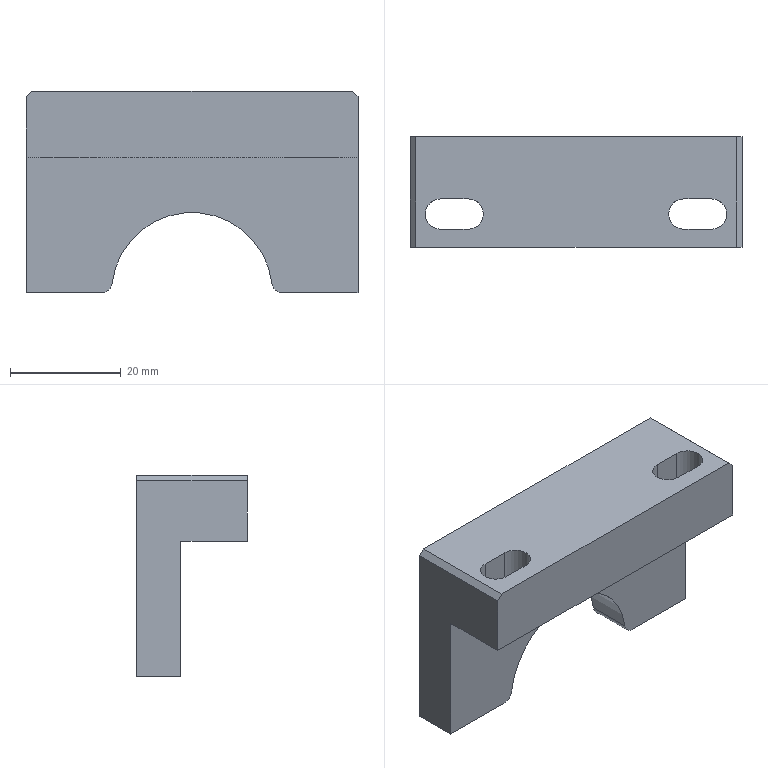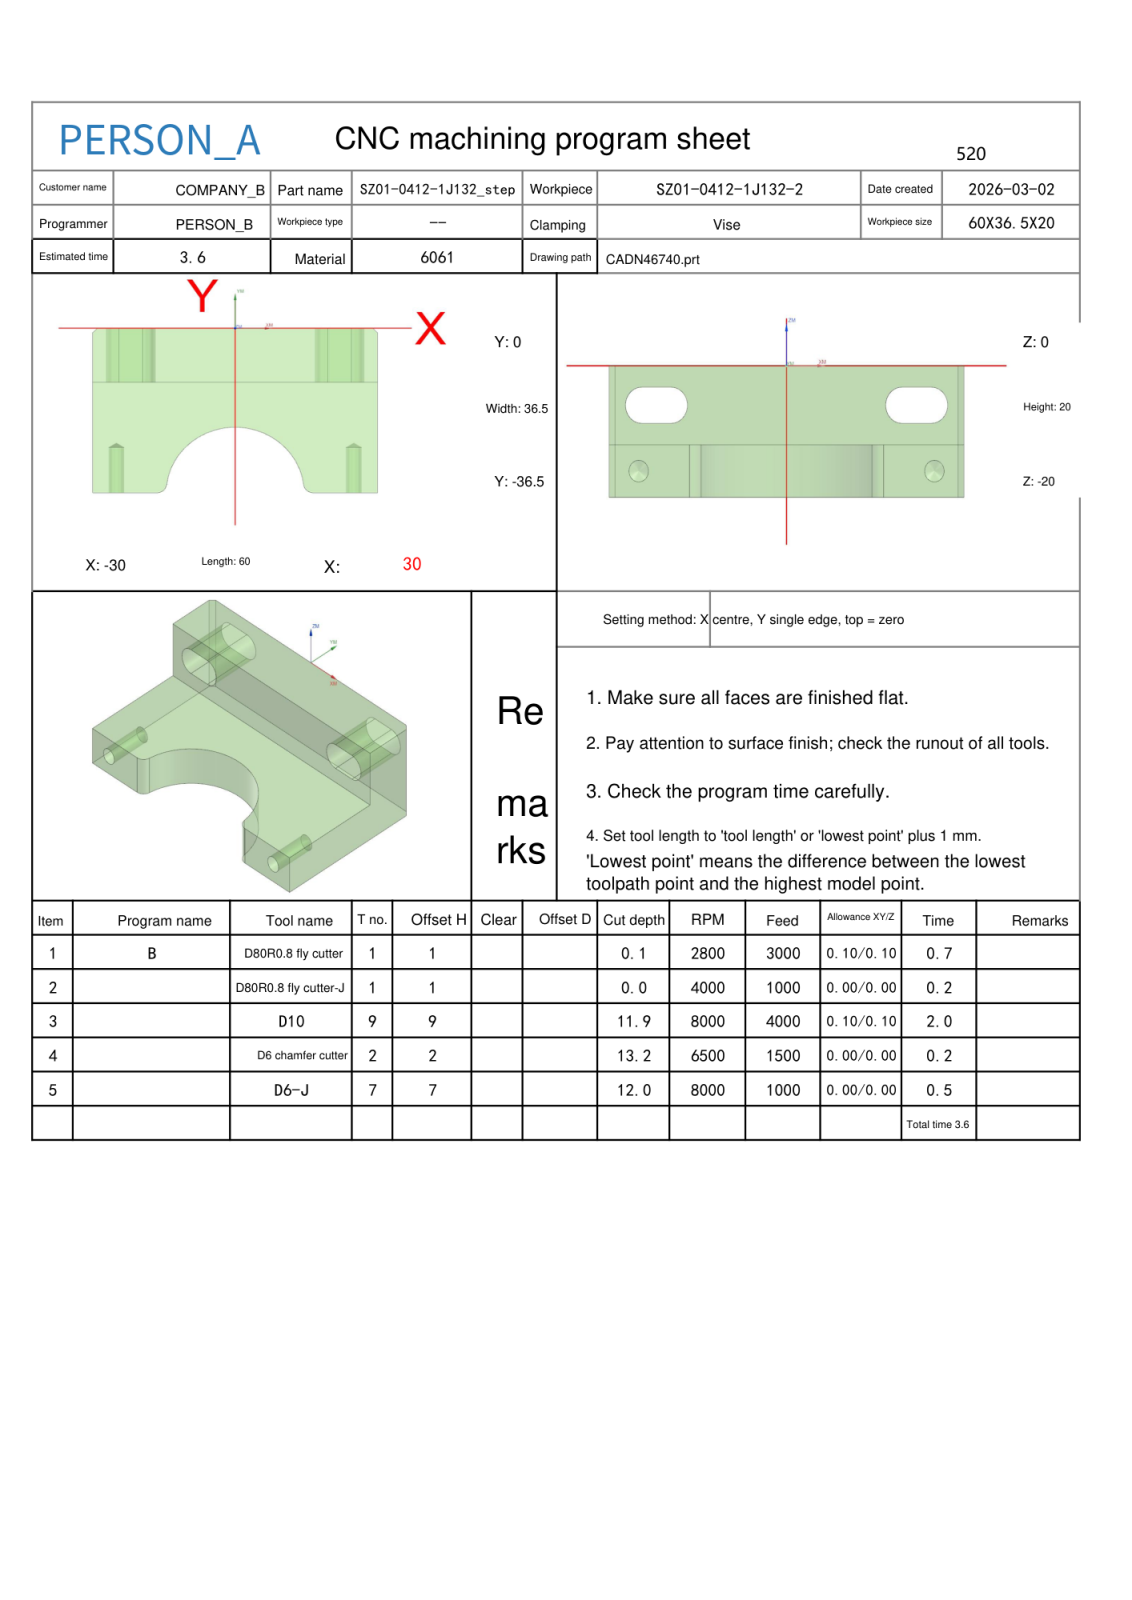NC program | NX | posted by the shop | part box 60 x 20 x 36.5 mm
Whole program, first 1625 of 1831 lines:
%
O0001
(Machine time: 4.61 MIN)
(===Total Tool:4===)
(T1=D80R0.8 fly cutter D=80.  R=0.8  D-  H01 Z=0.    )
(T9=D10     D=10.  R=0.   D-  H09 Z=-11.9 )
(T2=D6 chamfer cutter   D=6.   R=0.   D-  H02 Z=-13.2 )
(T7=D6-J    D=6.   R=0.   D7  H07 Z=-12.  )
G80 G90 G17 G49 G40
G91 G28 Z0
M01
N1 T01 M06
(D80R0.8 fly cutter  D=80. R=0.8 H=01 ce=0.10 di=0.10)
G00 G90 G54 X82.097 Y-18.25 M03 S2800
G43 H01 Z50.
M08
Z6.011
G01 Z4.011 F3000.
X70.097
X-70.097
X-82.097
Z6.011
G00 X82.097
Z5.522
G01 Z3.522
X70.097
X-70.097
X-82.097
Z5.522
G00 X82.097
Z5.033
G01 Z3.033
X70.097
X-70.097
X-82.097
Z5.033
G00 X82.097
Z4.544
G01 Z2.544
X70.097
X-70.097
X-82.097
Z4.544
G00 Z50.
X82.097
Z4.056
G01 Z2.056
X70.097
X-70.097
X-82.097
Z4.056
G00 Z50.
X82.097
Z3.567
G01 Z1.567
X70.097
X-70.097
X-82.097
Z3.567
G00 Z50.
X82.097
Z3.078
G01 Z1.078
X70.097
X-70.097
X-82.097
Z3.078
G00 Z50.
X82.097
Z2.589
G01 Z.589
X70.097
X-70.097
X-82.097
Z2.589
G00 Z50.
X82.097
Z2.1
G01 Z.1
X70.097
X-70.097
X-82.097
Z2.1
G00 Z50.
G91 G28 Z0.0
M05
M09
G91 G28 Z0.0
M01
N2 T01 M06
(D80R0.8 fly cutter-J  D=80. R=0.8 H=01 ce=0.00 di=0.00)
G00 G90 G54 X81.999 Y-18.25 M03 S4000
G43 H01 Z50.
M08
Z2.
G01 Z0.0 F1000.
X69.999
X-69.999
X-81.999
Z2.
G00 Z50.
G91 G28 Z0.0
M05
M09
G91 G28 Z0.0
M01
N3 T09 M06
(D10  D=10. R=0. H=09 ce=0.10 di=0.10)
G00 G90 G54 X38. Y-29.25 M03 S8000
G43 H09 Z14.5
M08
Z.905
G01 Z-.595 F4000.
X34.9
Y-41.4
X16.429
G02 X9.579 Y-35.334 I0.0 J6.9
G03 X0.0 Y-26.85 I-9.579 J-1.166
X-9.579 Y-35.334 I0.0 J-9.65
G02 X-16.429 Y-41.4 I-6.849 J.834
G01 X-34.9
Y-17.1
X-14.511
G02 X-13.511 Y-18.1 I0.0 J-1.
G01 X-13.522 Y-18.254
X-14.384 Y-23.787
X-14.396 Y-23.941
G03 X-13.954 Y-24.77 I1. J0.0
G02 X-13.512 Y-25.6 I-.558 J-.83
X-13.712 Y-26.199 I-1. J0.0
G03 X-16.81 Y-33.1 I13.712 J-10.301
G02 X-17.787 Y-33.9 I-.98 J.2
G01 X-26.402
G02 X-27.4 Y-32.902 I.002 J1.
G01 Y-25.598
G02 X-26.402 Y-24.6 I1. J-.002
G01 X-17.809
G03 X-16.834 Y-23.822 I0.0 J1.
G01 X-15.486 Y-17.879
G02 X-14.511 Y-17.1 I.975 J-.221
G01 X-.81
G02 X.189 Y-18.066 I0.0 J-1.
G01 X.205 Y-18.539
G03 X.764 Y-19.403 I.999 J.034
G02 X2.162 Y-21.647 I-1.102 J-2.244
X.134 Y-24.102 I-2.5 J0.0
G01 X-10.853 Y-26.214
G02 X-11.325 Y-26.259 I-.472 J2.455
X-13.825 Y-23.759 I0.0 J2.5
X-11.797 Y-21.304 I2.5 J0.0
G01 X-2.631 Y-19.542
G03 X-1.82 Y-18.581 I-.189 J.982
G01 X-1.81 Y-18.079
G02 X-.81 Y-17.1 I1. J-.021
G01 X.81
G02 X1.81 Y-18.079 I0.0 J-1.
G01 X1.82 Y-18.581
G03 X2.631 Y-19.542 I1. J.021
G01 X11.797 Y-21.304
G02 X13.825 Y-23.759 I-.472 J-2.455
X11.325 Y-26.259 I-2.5 J0.0
X10.853 Y-26.214 I0.0 J2.5
G01 X-.134 Y-24.102
G02 X-2.162 Y-21.647 I.472 J2.455
X-.764 Y-19.403 I2.5 J0.0
G03 X-.205 Y-18.539 I-.441 J.897
G01 X-.189 Y-18.066
G02 X.81 Y-17.1 I.999 J-.034
G01 X34.9
Y-26.215
G02 X34.455 Y-27.047 I-1. J0.0
G01 X27.845 Y-31.453
G03 X27.4 Y-32.285 I.555 J-.832
G01 Y-32.902
G02 X26.402 Y-33.9 I-1. J.002
G01 X17.787
G02 X16.81 Y-33.1 I.002 J1.
G03 X13.712 Y-26.199 I-16.81 J-3.4
G02 X13.512 Y-25.6 I.801 J.599
X14.511 Y-24.6 I1. J0.0
G01 X26.402
G02 X27.4 Y-25.598 I-.002 J-1.
G01 Y-29.25
Y-29.75
X38.
Z.905
G00 Y-29.25
Z.31
G01 Z-1.19
X34.9
Y-41.4
X16.429
G02 X9.579 Y-35.334 I0.0 J6.9
G03 X0.0 Y-26.85 I-9.579 J-1.166
X-9.579 Y-35.334 I0.0 J-9.65
G02 X-16.429 Y-41.4 I-6.849 J.834
G01 X-34.9
Y-17.1
X-14.511
G02 X-13.511 Y-18.1 I0.0 J-1.
G01 X-13.522 Y-18.254
X-14.384 Y-23.787
X-14.396 Y-23.941
G03 X-13.954 Y-24.77 I1. J0.0
G02 X-13.512 Y-25.6 I-.558 J-.83
X-13.712 Y-26.199 I-1. J0.0
G03 X-16.81 Y-33.1 I13.712 J-10.301
G02 X-17.787 Y-33.9 I-.98 J.2
G01 X-26.402
G02 X-27.4 Y-32.902 I.002 J1.
G01 Y-25.598
G02 X-26.402 Y-24.6 I1. J-.002
G01 X-17.809
G03 X-16.834 Y-23.822 I0.0 J1.
G01 X-15.486 Y-17.879
G02 X-14.511 Y-17.1 I.975 J-.221
G01 X-.81
G02 X.189 Y-18.066 I0.0 J-1.
G01 X.205 Y-18.539
G03 X.764 Y-19.403 I.999 J.034
G02 X2.162 Y-21.647 I-1.102 J-2.244
X.134 Y-24.102 I-2.5 J0.0
G01 X-10.853 Y-26.214
G02 X-11.325 Y-26.259 I-.472 J2.455
X-13.825 Y-23.759 I0.0 J2.5
X-11.797 Y-21.304 I2.5 J0.0
G01 X-2.631 Y-19.542
G03 X-1.82 Y-18.581 I-.189 J.982
G01 X-1.81 Y-18.079
G02 X-.81 Y-17.1 I1. J-.021
G01 X.81
G02 X1.81 Y-18.079 I0.0 J-1.
G01 X1.82 Y-18.581
G03 X2.631 Y-19.542 I1. J.021
G01 X11.797 Y-21.304
G02 X13.825 Y-23.759 I-.472 J-2.455
X11.325 Y-26.259 I-2.5 J0.0
X10.853 Y-26.214 I0.0 J2.5
G01 X-.134 Y-24.102
G02 X-2.162 Y-21.647 I.472 J2.455
X-.764 Y-19.403 I2.5 J0.0
G03 X-.205 Y-18.539 I-.441 J.897
G01 X-.189 Y-18.066
G02 X.81 Y-17.1 I.999 J-.034
G01 X34.9
Y-26.215
G02 X34.455 Y-27.047 I-1. J0.0
G01 X27.845 Y-31.453
G03 X27.4 Y-32.285 I.555 J-.832
G01 Y-32.902
G02 X26.402 Y-33.9 I-1. J.002
G01 X17.787
G02 X16.81 Y-33.1 I.002 J1.
G03 X13.712 Y-26.199 I-16.81 J-3.4
G02 X13.512 Y-25.6 I.801 J.599
X14.511 Y-24.6 I1. J0.0
G01 X26.402
G02 X27.4 Y-25.598 I-.002 J-1.
G01 Y-29.25
Y-29.75
X38.
Z.31
G00 Y-29.25
Z-.285
G01 Z-1.785
X34.9
Y-41.4
X16.429
G02 X9.579 Y-35.334 I0.0 J6.9
G03 X0.0 Y-26.85 I-9.579 J-1.166
X-9.579 Y-35.334 I0.0 J-9.65
G02 X-16.429 Y-41.4 I-6.849 J.834
G01 X-34.9
Y-17.1
X-14.511
G02 X-13.511 Y-18.1 I0.0 J-1.
G01 X-13.522 Y-18.254
X-14.384 Y-23.787
X-14.396 Y-23.941
G03 X-13.954 Y-24.77 I1. J0.0
G02 X-13.512 Y-25.6 I-.558 J-.83
X-13.712 Y-26.199 I-1. J0.0
G03 X-16.81 Y-33.1 I13.712 J-10.301
G02 X-17.787 Y-33.9 I-.98 J.2
G01 X-26.402
G02 X-27.4 Y-32.902 I.002 J1.
G01 Y-25.598
G02 X-26.402 Y-24.6 I1. J-.002
G01 X-17.809
G03 X-16.834 Y-23.822 I0.0 J1.
G01 X-15.486 Y-17.879
G02 X-14.511 Y-17.1 I.975 J-.221
G01 X-.81
G02 X.189 Y-18.066 I0.0 J-1.
G01 X.205 Y-18.539
G03 X.764 Y-19.403 I.999 J.034
G02 X2.162 Y-21.647 I-1.102 J-2.244
X.134 Y-24.102 I-2.5 J0.0
G01 X-10.853 Y-26.214
G02 X-11.325 Y-26.259 I-.472 J2.455
X-13.825 Y-23.759 I0.0 J2.5
X-11.797 Y-21.304 I2.5 J0.0
G01 X-2.631 Y-19.542
G03 X-1.82 Y-18.581 I-.189 J.982
G01 X-1.81 Y-18.079
G02 X-.81 Y-17.1 I1. J-.021
G01 X.81
G02 X1.81 Y-18.079 I0.0 J-1.
G01 X1.82 Y-18.581
G03 X2.631 Y-19.542 I1. J.021
G01 X11.797 Y-21.304
G02 X13.825 Y-23.759 I-.472 J-2.455
X11.325 Y-26.259 I-2.5 J0.0
X10.853 Y-26.214 I0.0 J2.5
G01 X-.134 Y-24.102
G02 X-2.162 Y-21.647 I.472 J2.455
X-.764 Y-19.403 I2.5 J0.0
G03 X-.205 Y-18.539 I-.441 J.897
G01 X-.189 Y-18.066
G02 X.81 Y-17.1 I.999 J-.034
G01 X34.9
Y-26.215
G02 X34.455 Y-27.047 I-1. J0.0
G01 X27.845 Y-31.453
G03 X27.4 Y-32.285 I.555 J-.832
G01 Y-32.902
G02 X26.402 Y-33.9 I-1. J.002
G01 X17.787
G02 X16.81 Y-33.1 I.002 J1.
G03 X13.712 Y-26.199 I-16.81 J-3.4
G02 X13.512 Y-25.6 I.801 J.599
X14.511 Y-24.6 I1. J0.0
G01 X26.402
G02 X27.4 Y-25.598 I-.002 J-1.
G01 Y-29.25
Y-29.75
X38.
Z-.285
G00 Y-29.25
Z-.88
G01 Z-2.38
X34.9
Y-41.4
X16.429
G02 X9.579 Y-35.334 I0.0 J6.9
G03 X0.0 Y-26.85 I-9.579 J-1.166
X-9.579 Y-35.334 I0.0 J-9.65
G02 X-16.429 Y-41.4 I-6.849 J.834
G01 X-34.9
Y-17.1
X-14.511
G02 X-13.511 Y-18.1 I0.0 J-1.
G01 X-13.522 Y-18.254
X-14.384 Y-23.787
X-14.396 Y-23.941
G03 X-13.954 Y-24.77 I1. J0.0
G02 X-13.512 Y-25.6 I-.558 J-.83
X-13.712 Y-26.199 I-1. J0.0
G03 X-16.81 Y-33.1 I13.712 J-10.301
G02 X-17.787 Y-33.9 I-.98 J.2
G01 X-26.402
G02 X-27.4 Y-32.902 I.002 J1.
G01 Y-25.598
G02 X-26.402 Y-24.6 I1. J-.002
G01 X-17.809
G03 X-16.834 Y-23.822 I0.0 J1.
G01 X-15.486 Y-17.879
G02 X-14.511 Y-17.1 I.975 J-.221
G01 X-.81
G02 X.189 Y-18.066 I0.0 J-1.
G01 X.205 Y-18.539
G03 X.764 Y-19.403 I.999 J.034
G02 X2.162 Y-21.647 I-1.102 J-2.244
X.134 Y-24.102 I-2.5 J0.0
G01 X-10.853 Y-26.214
G02 X-11.325 Y-26.259 I-.472 J2.455
X-13.825 Y-23.759 I0.0 J2.5
X-11.797 Y-21.304 I2.5 J0.0
G01 X-2.631 Y-19.542
G03 X-1.82 Y-18.581 I-.189 J.982
G01 X-1.81 Y-18.079
G02 X-.81 Y-17.1 I1. J-.021
G01 X.81
G02 X1.81 Y-18.079 I0.0 J-1.
G01 X1.82 Y-18.581
G03 X2.631 Y-19.542 I1. J.021
G01 X11.797 Y-21.304
G02 X13.825 Y-23.759 I-.472 J-2.455
X11.325 Y-26.259 I-2.5 J0.0
X10.853 Y-26.214 I0.0 J2.5
G01 X-.134 Y-24.102
G02 X-2.162 Y-21.647 I.472 J2.455
X-.764 Y-19.403 I2.5 J0.0
G03 X-.205 Y-18.539 I-.441 J.897
G01 X-.189 Y-18.066
G02 X.81 Y-17.1 I.999 J-.034
G01 X34.9
Y-26.215
G02 X34.455 Y-27.047 I-1. J0.0
G01 X27.845 Y-31.453
G03 X27.4 Y-32.285 I.555 J-.832
G01 Y-32.902
G02 X26.402 Y-33.9 I-1. J.002
G01 X17.787
G02 X16.81 Y-33.1 I.002 J1.
G03 X13.712 Y-26.199 I-16.81 J-3.4
G02 X13.512 Y-25.6 I.801 J.599
X14.511 Y-24.6 I1. J0.0
G01 X26.402
G02 X27.4 Y-25.598 I-.002 J-1.
G01 Y-29.25
Y-29.75
X38.
Z-.88
G00 Y-29.25
Z-1.475
G01 Z-2.975
X34.9
Y-41.4
X16.429
G02 X9.579 Y-35.334 I0.0 J6.9
G03 X0.0 Y-26.85 I-9.579 J-1.166
X-9.579 Y-35.334 I0.0 J-9.65
G02 X-16.429 Y-41.4 I-6.849 J.834
G01 X-34.9
Y-17.1
X-14.511
G02 X-13.511 Y-18.1 I0.0 J-1.
G01 X-13.522 Y-18.254
X-14.384 Y-23.787
X-14.396 Y-23.941
G03 X-13.954 Y-24.77 I1. J0.0
G02 X-13.512 Y-25.6 I-.558 J-.83
X-13.712 Y-26.199 I-1. J0.0
G03 X-16.81 Y-33.1 I13.712 J-10.301
G02 X-17.787 Y-33.9 I-.98 J.2
G01 X-26.402
G02 X-27.4 Y-32.902 I.002 J1.
G01 Y-25.598
G02 X-26.402 Y-24.6 I1. J-.002
G01 X-17.809
G03 X-16.834 Y-23.822 I0.0 J1.
G01 X-15.486 Y-17.879
G02 X-14.511 Y-17.1 I.975 J-.221
G01 X-.81
G02 X.189 Y-18.066 I0.0 J-1.
G01 X.205 Y-18.539
G03 X.764 Y-19.403 I.999 J.034
G02 X2.162 Y-21.647 I-1.102 J-2.244
X.134 Y-24.102 I-2.5 J0.0
G01 X-10.853 Y-26.214
G02 X-11.325 Y-26.259 I-.472 J2.455
X-13.825 Y-23.759 I0.0 J2.5
X-11.797 Y-21.304 I2.5 J0.0
G01 X-2.631 Y-19.542
G03 X-1.82 Y-18.581 I-.189 J.982
G01 X-1.81 Y-18.079
G02 X-.81 Y-17.1 I1. J-.021
G01 X.81
G02 X1.81 Y-18.079 I0.0 J-1.
G01 X1.82 Y-18.581
G03 X2.631 Y-19.542 I1. J.021
G01 X11.797 Y-21.304
G02 X13.825 Y-23.759 I-.472 J-2.455
X11.325 Y-26.259 I-2.5 J0.0
X10.853 Y-26.214 I0.0 J2.5
G01 X-.134 Y-24.102
G02 X-2.162 Y-21.647 I.472 J2.455
X-.764 Y-19.403 I2.5 J0.0
G03 X-.205 Y-18.539 I-.441 J.897
G01 X-.189 Y-18.066
G02 X.81 Y-17.1 I.999 J-.034
G01 X34.9
Y-26.215
G02 X34.455 Y-27.047 I-1. J0.0
G01 X27.845 Y-31.453
G03 X27.4 Y-32.285 I.555 J-.832
G01 Y-32.902
G02 X26.402 Y-33.9 I-1. J.002
G01 X17.787
G02 X16.81 Y-33.1 I.002 J1.
G03 X13.712 Y-26.199 I-16.81 J-3.4
G02 X13.512 Y-25.6 I.801 J.599
X14.511 Y-24.6 I1. J0.0
G01 X26.402
G02 X27.4 Y-25.598 I-.002 J-1.
G01 Y-29.25
Y-29.75
X38.
Z-1.475
G00 Y-29.25
Z-2.07
G01 Z-3.57
X34.9
Y-41.4
X16.429
G02 X9.579 Y-35.334 I0.0 J6.9
G03 X0.0 Y-26.85 I-9.579 J-1.166
X-9.579 Y-35.334 I0.0 J-9.65
G02 X-16.429 Y-41.4 I-6.849 J.834
G01 X-34.9
Y-17.1
X-14.511
G02 X-13.511 Y-18.1 I0.0 J-1.
G01 X-13.522 Y-18.254
X-14.384 Y-23.787
X-14.396 Y-23.941
G03 X-13.954 Y-24.77 I1. J0.0
G02 X-13.512 Y-25.6 I-.558 J-.83
X-13.712 Y-26.199 I-1. J0.0
G03 X-16.81 Y-33.1 I13.712 J-10.301
G02 X-17.787 Y-33.9 I-.98 J.2
G01 X-26.402
G02 X-27.4 Y-32.902 I.002 J1.
G01 Y-25.598
G02 X-26.402 Y-24.6 I1. J-.002
G01 X-17.809
G03 X-16.834 Y-23.822 I0.0 J1.
G01 X-15.486 Y-17.879
G02 X-14.511 Y-17.1 I.975 J-.221
G01 X-.81
G02 X.189 Y-18.066 I0.0 J-1.
G01 X.205 Y-18.539
G03 X.764 Y-19.403 I.999 J.034
G02 X2.162 Y-21.647 I-1.102 J-2.244
X.134 Y-24.102 I-2.5 J0.0
G01 X-10.853 Y-26.214
G02 X-11.325 Y-26.259 I-.472 J2.455
X-13.825 Y-23.759 I0.0 J2.5
X-11.797 Y-21.304 I2.5 J0.0
G01 X-2.631 Y-19.542
G03 X-1.82 Y-18.581 I-.189 J.982
G01 X-1.81 Y-18.079
G02 X-.81 Y-17.1 I1. J-.021
G01 X.81
G02 X1.81 Y-18.079 I0.0 J-1.
G01 X1.82 Y-18.581
G03 X2.631 Y-19.542 I1. J.021
G01 X11.797 Y-21.304
G02 X13.825 Y-23.759 I-.472 J-2.455
X11.325 Y-26.259 I-2.5 J0.0
X10.853 Y-26.214 I0.0 J2.5
G01 X-.134 Y-24.102
G02 X-2.162 Y-21.647 I.472 J2.455
X-.764 Y-19.403 I2.5 J0.0
G03 X-.205 Y-18.539 I-.441 J.897
G01 X-.189 Y-18.066
G02 X.81 Y-17.1 I.999 J-.034
G01 X34.9
Y-26.215
G02 X34.455 Y-27.047 I-1. J0.0
G01 X27.845 Y-31.453
G03 X27.4 Y-32.285 I.555 J-.832
G01 Y-32.902
G02 X26.402 Y-33.9 I-1. J.002
G01 X17.787
G02 X16.81 Y-33.1 I.002 J1.
G03 X13.712 Y-26.199 I-16.81 J-3.4
G02 X13.512 Y-25.6 I.801 J.599
X14.511 Y-24.6 I1. J0.0
G01 X26.402
G02 X27.4 Y-25.598 I-.002 J-1.
G01 Y-29.25
Y-29.75
X38.
Z-2.07
G00 Y-29.25
Z-2.665
G01 Z-4.165
X34.9
Y-41.4
X16.429
G02 X9.579 Y-35.334 I0.0 J6.9
G03 X0.0 Y-26.85 I-9.579 J-1.166
X-9.579 Y-35.334 I0.0 J-9.65
G02 X-16.429 Y-41.4 I-6.849 J.834
G01 X-34.9
Y-17.1
X-14.511
G02 X-13.511 Y-18.1 I0.0 J-1.
G01 X-13.522 Y-18.254
X-14.384 Y-23.787
X-14.396 Y-23.941
G03 X-13.954 Y-24.77 I1. J0.0
G02 X-13.512 Y-25.6 I-.558 J-.83
X-13.712 Y-26.199 I-1. J0.0
G03 X-16.81 Y-33.1 I13.712 J-10.301
G02 X-17.787 Y-33.9 I-.98 J.2
G01 X-26.402
G02 X-27.4 Y-32.902 I.002 J1.
G01 Y-25.598
G02 X-26.402 Y-24.6 I1. J-.002
G01 X-17.809
G03 X-16.834 Y-23.822 I0.0 J1.
G01 X-15.486 Y-17.879
G02 X-14.511 Y-17.1 I.975 J-.221
G01 X-.81
G02 X.189 Y-18.066 I0.0 J-1.
G01 X.205 Y-18.539
G03 X.764 Y-19.403 I.999 J.034
G02 X2.162 Y-21.647 I-1.102 J-2.244
X.134 Y-24.102 I-2.5 J0.0
G01 X-10.853 Y-26.214
G02 X-11.325 Y-26.259 I-.472 J2.455
X-13.825 Y-23.759 I0.0 J2.5
X-11.797 Y-21.304 I2.5 J0.0
G01 X-2.631 Y-19.542
G03 X-1.82 Y-18.581 I-.189 J.982
G01 X-1.81 Y-18.079
G02 X-.81 Y-17.1 I1. J-.021
G01 X.81
G02 X1.81 Y-18.079 I0.0 J-1.
G01 X1.82 Y-18.581
G03 X2.631 Y-19.542 I1. J.021
G01 X11.797 Y-21.304
G02 X13.825 Y-23.759 I-.472 J-2.455
X11.325 Y-26.259 I-2.5 J0.0
X10.853 Y-26.214 I0.0 J2.5
G01 X-.134 Y-24.102
G02 X-2.162 Y-21.647 I.472 J2.455
X-.764 Y-19.403 I2.5 J0.0
G03 X-.205 Y-18.539 I-.441 J.897
G01 X-.189 Y-18.066
G02 X.81 Y-17.1 I.999 J-.034
G01 X34.9
Y-26.215
G02 X34.455 Y-27.047 I-1. J0.0
G01 X27.845 Y-31.453
G03 X27.4 Y-32.285 I.555 J-.832
G01 Y-32.902
G02 X26.402 Y-33.9 I-1. J.002
G01 X17.787
G02 X16.81 Y-33.1 I.002 J1.
G03 X13.712 Y-26.199 I-16.81 J-3.4
G02 X13.512 Y-25.6 I.801 J.599
X14.511 Y-24.6 I1. J0.0
G01 X26.402
G02 X27.4 Y-25.598 I-.002 J-1.
G01 Y-29.25
Y-29.75
X38.
Z-2.665
G00 Y-29.25
Z-3.26
G01 Z-4.76
X34.9
Y-41.4
X16.429
G02 X9.579 Y-35.334 I0.0 J6.9
G03 X0.0 Y-26.85 I-9.579 J-1.166
X-9.579 Y-35.334 I0.0 J-9.65
G02 X-16.429 Y-41.4 I-6.849 J.834
G01 X-34.9
Y-17.1
X-14.511
G02 X-13.511 Y-18.1 I0.0 J-1.
G01 X-13.522 Y-18.254
X-14.384 Y-23.787
X-14.396 Y-23.941
G03 X-13.954 Y-24.77 I1. J0.0
G02 X-13.512 Y-25.6 I-.558 J-.83
X-13.712 Y-26.199 I-1. J0.0
G03 X-16.81 Y-33.1 I13.712 J-10.301
G02 X-17.787 Y-33.9 I-.98 J.2
G01 X-26.402
G02 X-27.4 Y-32.902 I.002 J1.
G01 Y-25.598
G02 X-26.402 Y-24.6 I1. J-.002
G01 X-17.809
G03 X-16.834 Y-23.822 I0.0 J1.
G01 X-15.486 Y-17.879
G02 X-14.511 Y-17.1 I.975 J-.221
G01 X-.81
G02 X.189 Y-18.066 I0.0 J-1.
G01 X.205 Y-18.539
G03 X.764 Y-19.403 I.999 J.034
G02 X2.162 Y-21.647 I-1.102 J-2.244
X.134 Y-24.102 I-2.5 J0.0
G01 X-10.853 Y-26.214
G02 X-11.325 Y-26.259 I-.472 J2.455
X-13.825 Y-23.759 I0.0 J2.5
X-11.797 Y-21.304 I2.5 J0.0
G01 X-2.631 Y-19.542
G03 X-1.82 Y-18.581 I-.189 J.982
G01 X-1.81 Y-18.079
G02 X-.81 Y-17.1 I1. J-.021
G01 X.81
G02 X1.81 Y-18.079 I0.0 J-1.
G01 X1.82 Y-18.581
G03 X2.631 Y-19.542 I1. J.021
G01 X11.797 Y-21.304
G02 X13.825 Y-23.759 I-.472 J-2.455
X11.325 Y-26.259 I-2.5 J0.0
X10.853 Y-26.214 I0.0 J2.5
G01 X-.134 Y-24.102
G02 X-2.162 Y-21.647 I.472 J2.455
X-.764 Y-19.403 I2.5 J0.0
G03 X-.205 Y-18.539 I-.441 J.897
G01 X-.189 Y-18.066
G02 X.81 Y-17.1 I.999 J-.034
G01 X34.9
Y-26.215
G02 X34.455 Y-27.047 I-1. J0.0
G01 X27.845 Y-31.453
G03 X27.4 Y-32.285 I.555 J-.832
G01 Y-32.902
G02 X26.402 Y-33.9 I-1. J.002
G01 X17.787
G02 X16.81 Y-33.1 I.002 J1.
G03 X13.712 Y-26.199 I-16.81 J-3.4
G02 X13.512 Y-25.6 I.801 J.599
X14.511 Y-24.6 I1. J0.0
G01 X26.402
G02 X27.4 Y-25.598 I-.002 J-1.
G01 Y-29.25
Y-29.75
X38.
Z-3.26
G00 Y-29.25
Z-3.855
G01 Z-5.355
X34.9
Y-41.4
X16.429
G02 X9.579 Y-35.334 I0.0 J6.9
G03 X0.0 Y-26.85 I-9.579 J-1.166
X-9.579 Y-35.334 I0.0 J-9.65
G02 X-16.429 Y-41.4 I-6.849 J.834
G01 X-34.9
Y-17.1
X-14.511
G02 X-13.511 Y-18.1 I0.0 J-1.
G01 X-13.522 Y-18.254
X-14.384 Y-23.787
X-14.396 Y-23.941
G03 X-13.954 Y-24.77 I1. J0.0
G02 X-13.512 Y-25.6 I-.558 J-.83
X-13.712 Y-26.199 I-1. J0.0
G03 X-16.81 Y-33.1 I13.712 J-10.301
G02 X-17.787 Y-33.9 I-.98 J.2
G01 X-26.402
G02 X-27.4 Y-32.902 I.002 J1.
G01 Y-25.598
G02 X-26.402 Y-24.6 I1. J-.002
G01 X-17.809
G03 X-16.834 Y-23.822 I0.0 J1.
G01 X-15.486 Y-17.879
G02 X-14.511 Y-17.1 I.975 J-.221
G01 X-.81
G02 X.189 Y-18.066 I0.0 J-1.
G01 X.205 Y-18.539
G03 X.764 Y-19.403 I.999 J.034
G02 X2.162 Y-21.647 I-1.102 J-2.244
X.134 Y-24.102 I-2.5 J0.0
G01 X-10.853 Y-26.214
G02 X-11.325 Y-26.259 I-.472 J2.455
X-13.825 Y-23.759 I0.0 J2.5
X-11.797 Y-21.304 I2.5 J0.0
G01 X-2.631 Y-19.542
G03 X-1.82 Y-18.581 I-.189 J.982
G01 X-1.81 Y-18.079
G02 X-.81 Y-17.1 I1. J-.021
G01 X.81
G02 X1.81 Y-18.079 I0.0 J-1.
G01 X1.82 Y-18.581
G03 X2.631 Y-19.542 I1. J.021
G01 X11.797 Y-21.304
G02 X13.825 Y-23.759 I-.472 J-2.455
X11.325 Y-26.259 I-2.5 J0.0
X10.853 Y-26.214 I0.0 J2.5
G01 X-.134 Y-24.102
G02 X-2.162 Y-21.647 I.472 J2.455
X-.764 Y-19.403 I2.5 J0.0
G03 X-.205 Y-18.539 I-.441 J.897
G01 X-.189 Y-18.066
G02 X.81 Y-17.1 I.999 J-.034
G01 X34.9
Y-26.215
G02 X34.455 Y-27.047 I-1. J0.0
G01 X27.845 Y-31.453
G03 X27.4 Y-32.285 I.555 J-.832
G01 Y-32.902
G02 X26.402 Y-33.9 I-1. J.002
G01 X17.787
G02 X16.81 Y-33.1 I.002 J1.
G03 X13.712 Y-26.199 I-16.81 J-3.4
G02 X13.512 Y-25.6 I.801 J.599
X14.511 Y-24.6 I1. J0.0
G01 X26.402
G02 X27.4 Y-25.598 I-.002 J-1.
G01 Y-29.25
Y-29.75
X38.
Z-3.855
G00 Y-29.25
Z-4.45
G01 Z-5.95
X34.9
Y-41.4
X16.429
G02 X9.579 Y-35.334 I0.0 J6.9
G03 X0.0 Y-26.85 I-9.579 J-1.166
X-9.579 Y-35.334 I0.0 J-9.65
G02 X-16.429 Y-41.4 I-6.849 J.834
G01 X-34.9
Y-17.1
X-14.511
G02 X-13.511 Y-18.1 I0.0 J-1.
G01 X-13.522 Y-18.254
X-14.384 Y-23.787
X-14.396 Y-23.941
G03 X-13.954 Y-24.77 I1. J0.0
G02 X-13.512 Y-25.6 I-.558 J-.83
X-13.712 Y-26.199 I-1. J0.0
G03 X-16.81 Y-33.1 I13.712 J-10.301
G02 X-17.787 Y-33.9 I-.98 J.2
G01 X-26.402
G02 X-27.4 Y-32.902 I.002 J1.
G01 Y-25.598
G02 X-26.402 Y-24.6 I1. J-.002
G01 X-17.809
G03 X-16.834 Y-23.822 I0.0 J1.
G01 X-15.486 Y-17.879
G02 X-14.511 Y-17.1 I.975 J-.221
G01 X-.81
G02 X.189 Y-18.066 I0.0 J-1.
G01 X.205 Y-18.539
G03 X.764 Y-19.403 I.999 J.034
G02 X2.162 Y-21.647 I-1.102 J-2.244
X.134 Y-24.102 I-2.5 J0.0
G01 X-10.853 Y-26.214
G02 X-11.325 Y-26.259 I-.472 J2.455
X-13.825 Y-23.759 I0.0 J2.5
X-11.797 Y-21.304 I2.5 J0.0
G01 X-2.631 Y-19.542
G03 X-1.82 Y-18.581 I-.189 J.982
G01 X-1.81 Y-18.079
G02 X-.81 Y-17.1 I1. J-.021
G01 X.81
G02 X1.81 Y-18.079 I0.0 J-1.
G01 X1.82 Y-18.581
G03 X2.631 Y-19.542 I1. J.021
G01 X11.797 Y-21.304
G02 X13.825 Y-23.759 I-.472 J-2.455
X11.325 Y-26.259 I-2.5 J0.0
X10.853 Y-26.214 I0.0 J2.5
G01 X-.134 Y-24.102
G02 X-2.162 Y-21.647 I.472 J2.455
X-.764 Y-19.403 I2.5 J0.0
G03 X-.205 Y-18.539 I-.441 J.897
G01 X-.189 Y-18.066
G02 X.81 Y-17.1 I.999 J-.034
G01 X34.9
Y-26.215
G02 X34.455 Y-27.047 I-1. J0.0
G01 X27.845 Y-31.453
G03 X27.4 Y-32.285 I.555 J-.832
G01 Y-32.902
G02 X26.402 Y-33.9 I-1. J.002
G01 X17.787
G02 X16.81 Y-33.1 I.002 J1.
G03 X13.712 Y-26.199 I-16.81 J-3.4
G02 X13.512 Y-25.6 I.801 J.599
X14.511 Y-24.6 I1. J0.0
G01 X26.402
G02 X27.4 Y-25.598 I-.002 J-1.
G01 Y-29.25
Y-29.75
X38.
Z-4.45
G00 Y-29.25
Z-5.045
G01 Z-6.545
X34.9
Y-41.4
X16.429
G02 X9.579 Y-35.334 I0.0 J6.9
G03 X0.0 Y-26.85 I-9.579 J-1.166
X-9.579 Y-35.334 I0.0 J-9.65
G02 X-16.429 Y-41.4 I-6.849 J.834
G01 X-34.9
Y-17.1
X-14.511
G02 X-13.511 Y-18.1 I0.0 J-1.
G01 X-13.522 Y-18.254
X-14.384 Y-23.787
X-14.396 Y-23.941
G03 X-13.954 Y-24.77 I1. J0.0
G02 X-13.512 Y-25.6 I-.558 J-.83
X-13.712 Y-26.199 I-1. J0.0
G03 X-16.81 Y-33.1 I13.712 J-10.301
G02 X-17.787 Y-33.9 I-.98 J.2
G01 X-26.402
G02 X-27.4 Y-32.902 I.002 J1.
G01 Y-25.598
G02 X-26.402 Y-24.6 I1. J-.002
G01 X-17.809
G03 X-16.834 Y-23.822 I0.0 J1.
G01 X-15.486 Y-17.879
G02 X-14.511 Y-17.1 I.975 J-.221
G01 X-.81
G02 X.189 Y-18.066 I0.0 J-1.
G01 X.205 Y-18.539
G03 X.764 Y-19.403 I.999 J.034
G02 X2.162 Y-21.647 I-1.102 J-2.244
X.134 Y-24.102 I-2.5 J0.0
G01 X-10.853 Y-26.214
G02 X-11.325 Y-26.259 I-.472 J2.455
X-13.825 Y-23.759 I0.0 J2.5
X-11.797 Y-21.304 I2.5 J0.0
G01 X-2.631 Y-19.542
G03 X-1.82 Y-18.581 I-.189 J.982
G01 X-1.81 Y-18.079
G02 X-.81 Y-17.1 I1. J-.021
G01 X.81
G02 X1.81 Y-18.079 I0.0 J-1.
G01 X1.82 Y-18.581
G03 X2.631 Y-19.542 I1. J.021
G01 X11.797 Y-21.304
G02 X13.825 Y-23.759 I-.472 J-2.455
X11.325 Y-26.259 I-2.5 J0.0
X10.853 Y-26.214 I0.0 J2.5
G01 X-.134 Y-24.102
G02 X-2.162 Y-21.647 I.472 J2.455
X-.764 Y-19.403 I2.5 J0.0
G03 X-.205 Y-18.539 I-.441 J.897
G01 X-.189 Y-18.066
G02 X.81 Y-17.1 I.999 J-.034
G01 X34.9
Y-26.215
G02 X34.455 Y-27.047 I-1. J0.0
G01 X27.845 Y-31.453
G03 X27.4 Y-32.285 I.555 J-.832
G01 Y-32.902
G02 X26.402 Y-33.9 I-1. J.002
G01 X17.787
G02 X16.81 Y-33.1 I.002 J1.
G03 X13.712 Y-26.199 I-16.81 J-3.4
G02 X13.512 Y-25.6 I.801 J.599
X14.511 Y-24.6 I1. J0.0
G01 X26.402
G02 X27.4 Y-25.598 I-.002 J-1.
G01 Y-29.25
Y-29.75
X38.
Z-5.045
G00 Y-29.25
Z-5.64
G01 Z-7.14
X34.9
Y-41.4
X16.429
G02 X9.579 Y-35.334 I0.0 J6.9
G03 X0.0 Y-26.85 I-9.579 J-1.166
X-9.579 Y-35.334 I0.0 J-9.65
G02 X-16.429 Y-41.4 I-6.849 J.834
G01 X-34.9
Y-17.1
X-14.511
G02 X-13.511 Y-18.1 I0.0 J-1.
G01 X-13.522 Y-18.254
X-14.384 Y-23.787
X-14.396 Y-23.941
G03 X-13.954 Y-24.77 I1. J0.0
G02 X-13.512 Y-25.6 I-.558 J-.83
X-13.712 Y-26.199 I-1. J0.0
G03 X-16.81 Y-33.1 I13.712 J-10.301
G02 X-17.787 Y-33.9 I-.98 J.2
G01 X-26.402
G02 X-27.4 Y-32.902 I.002 J1.
G01 Y-25.598
G02 X-26.402 Y-24.6 I1. J-.002
G01 X-17.809
G03 X-16.834 Y-23.822 I0.0 J1.
G01 X-15.486 Y-17.879
G02 X-14.511 Y-17.1 I.975 J-.221
G01 X-.81
G02 X.189 Y-18.066 I0.0 J-1.
G01 X.205 Y-18.539
G03 X.764 Y-19.403 I.999 J.034
G02 X2.162 Y-21.647 I-1.102 J-2.244
X.134 Y-24.102 I-2.5 J0.0
G01 X-10.853 Y-26.214
G02 X-11.325 Y-26.259 I-.472 J2.455
X-13.825 Y-23.759 I0.0 J2.5
X-11.797 Y-21.304 I2.5 J0.0
G01 X-2.631 Y-19.542
G03 X-1.82 Y-18.581 I-.189 J.982
G01 X-1.81 Y-18.079
G02 X-.81 Y-17.1 I1. J-.021
G01 X.81
G02 X1.81 Y-18.079 I0.0 J-1.
G01 X1.82 Y-18.581
G03 X2.631 Y-19.542 I1. J.021
G01 X11.797 Y-21.304
G02 X13.825 Y-23.759 I-.472 J-2.455
X11.325 Y-26.259 I-2.5 J0.0
X10.853 Y-26.214 I0.0 J2.5
G01 X-.134 Y-24.102
G02 X-2.162 Y-21.647 I.472 J2.455
X-.764 Y-19.403 I2.5 J0.0
G03 X-.205 Y-18.539 I-.441 J.897
G01 X-.189 Y-18.066
G02 X.81 Y-17.1 I.999 J-.034
G01 X34.9
Y-26.215
G02 X34.455 Y-27.047 I-1. J0.0
G01 X27.845 Y-31.453
G03 X27.4 Y-32.285 I.555 J-.832
G01 Y-32.902
G02 X26.402 Y-33.9 I-1. J.002
G01 X17.787
G02 X16.81 Y-33.1 I.002 J1.
G03 X13.712 Y-26.199 I-16.81 J-3.4
G02 X13.512 Y-25.6 I.801 J.599
X14.511 Y-24.6 I1. J0.0
G01 X26.402
G02 X27.4 Y-25.598 I-.002 J-1.
G01 Y-29.25
Y-29.75
X38.
Z-5.64
G00 Y-29.25
Z-6.235
G01 Z-7.735
X34.9
Y-41.4
X16.429
G02 X9.579 Y-35.334 I0.0 J6.9
G03 X0.0 Y-26.85 I-9.579 J-1.166
X-9.579 Y-35.334 I0.0 J-9.65
G02 X-16.429 Y-41.4 I-6.849 J.834
G01 X-34.9
Y-17.1
X-14.511
G02 X-13.511 Y-18.1 I0.0 J-1.
G01 X-13.522 Y-18.254
X-14.384 Y-23.787
X-14.396 Y-23.941
G03 X-13.954 Y-24.77 I1. J0.0
G02 X-13.512 Y-25.6 I-.558 J-.83
X-13.712 Y-26.199 I-1. J0.0
G03 X-16.81 Y-33.1 I13.712 J-10.301
G02 X-17.787 Y-33.9 I-.98 J.2
G01 X-26.402
G02 X-27.4 Y-32.902 I.002 J1.
G01 Y-25.598
G02 X-26.402 Y-24.6 I1. J-.002
G01 X-17.809
G03 X-16.834 Y-23.822 I0.0 J1.
G01 X-15.486 Y-17.879
G02 X-14.511 Y-17.1 I.975 J-.221
G01 X-.81
G02 X.189 Y-18.066 I0.0 J-1.
G01 X.205 Y-18.539
G03 X.764 Y-19.403 I.999 J.034
G02 X2.162 Y-21.647 I-1.102 J-2.244
X.134 Y-24.102 I-2.5 J0.0
G01 X-10.853 Y-26.214
G02 X-11.325 Y-26.259 I-.472 J2.455
X-13.825 Y-23.759 I0.0 J2.5
X-11.797 Y-21.304 I2.5 J0.0
G01 X-2.631 Y-19.542
G03 X-1.82 Y-18.581 I-.189 J.982
G01 X-1.81 Y-18.079
G02 X-.81 Y-17.1 I1. J-.021
G01 X.81
G02 X1.81 Y-18.079 I0.0 J-1.
G01 X1.82 Y-18.581
G03 X2.631 Y-19.542 I1. J.021
G01 X11.797 Y-21.304
G02 X13.825 Y-23.759 I-.472 J-2.455
X11.325 Y-26.259 I-2.5 J0.0
X10.853 Y-26.214 I0.0 J2.5
G01 X-.134 Y-24.102
G02 X-2.162 Y-21.647 I.472 J2.455
X-.764 Y-19.403 I2.5 J0.0
G03 X-.205 Y-18.539 I-.441 J.897
G01 X-.189 Y-18.066
G02 X.81 Y-17.1 I.999 J-.034
G01 X34.9
Y-26.215
G02 X34.455 Y-27.047 I-1. J0.0
G01 X27.845 Y-31.453
G03 X27.4 Y-32.285 I.555 J-.832
G01 Y-32.902
G02 X26.402 Y-33.9 I-1. J.002
G01 X17.787
G02 X16.81 Y-33.1 I.002 J1.
G03 X13.712 Y-26.199 I-16.81 J-3.4
G02 X13.512 Y-25.6 I.801 J.599
X14.511 Y-24.6 I1. J0.0
G01 X26.402
G02 X27.4 Y-25.598 I-.002 J-1.
G01 Y-29.25
Y-29.75
X38.
Z-6.235
G00 Y-29.25
Z-6.83
G01 Z-8.33
X34.9
Y-41.4
X16.429
G02 X9.579 Y-35.334 I0.0 J6.9
G03 X0.0 Y-26.85 I-9.579 J-1.166
X-9.579 Y-35.334 I0.0 J-9.65
G02 X-16.429 Y-41.4 I-6.849 J.834
G01 X-34.9
Y-17.1
X-14.511
G02 X-13.511 Y-18.1 I0.0 J-1.
G01 X-13.522 Y-18.254
X-14.384 Y-23.787
X-14.396 Y-23.941
G03 X-13.954 Y-24.77 I1. J0.0
G02 X-13.512 Y-25.6 I-.558 J-.83
X-13.712 Y-26.199 I-1. J0.0
G03 X-16.81 Y-33.1 I13.712 J-10.301
G02 X-17.787 Y-33.9 I-.98 J.2
G01 X-26.402
G02 X-27.4 Y-32.902 I.002 J1.
G01 Y-25.598
G02 X-26.402 Y-24.6 I1. J-.002
G01 X-17.809
G03 X-16.834 Y-23.822 I0.0 J1.
G01 X-15.486 Y-17.879
G02 X-14.511 Y-17.1 I.975 J-.221
G01 X-.81
G02 X.189 Y-18.066 I0.0 J-1.
G01 X.205 Y-18.539
G03 X.764 Y-19.403 I.999 J.034
G02 X2.162 Y-21.647 I-1.102 J-2.244
X.134 Y-24.102 I-2.5 J0.0
G01 X-10.853 Y-26.214
G02 X-11.325 Y-26.259 I-.472 J2.455
X-13.825 Y-23.759 I0.0 J2.5
X-11.797 Y-21.304 I2.5 J0.0
G01 X-2.631 Y-19.542
G03 X-1.82 Y-18.581 I-.189 J.982
G01 X-1.81 Y-18.079
G02 X-.81 Y-17.1 I1. J-.021
G01 X.81
G02 X1.81 Y-18.079 I0.0 J-1.
G01 X1.82 Y-18.581
G03 X2.631 Y-19.542 I1. J.021
G01 X11.797 Y-21.304
G02 X13.825 Y-23.759 I-.472 J-2.455
X11.325 Y-26.259 I-2.5 J0.0
X10.853 Y-26.214 I0.0 J2.5
G01 X-.134 Y-24.102
G02 X-2.162 Y-21.647 I.472 J2.455
X-.764 Y-19.403 I2.5 J0.0
G03 X-.205 Y-18.539 I-.441 J.897
G01 X-.189 Y-18.066
G02 X.81 Y-17.1 I.999 J-.034
G01 X34.9
Y-26.215
G02 X34.455 Y-27.047 I-1. J0.0
G01 X27.845 Y-31.453
G03 X27.4 Y-32.285 I.555 J-.832
G01 Y-32.902
G02 X26.402 Y-33.9 I-1. J.002
G01 X17.787
G02 X16.81 Y-33.1 I.002 J1.
G03 X13.712 Y-26.199 I-16.81 J-3.4
G02 X13.512 Y-25.6 I.801 J.599
X14.511 Y-24.6 I1. J0.0
G01 X26.402
G02 X27.4 Y-25.598 I-.002 J-1.
G01 Y-29.25
Y-29.75
X38.
Z-6.83
G00 Y-29.25
Z-7.425
G01 Z-8.925
X34.9
Y-41.4
X16.429
G02 X9.579 Y-35.334 I0.0 J6.9
G03 X0.0 Y-26.85 I-9.579 J-1.166
X-9.579 Y-35.334 I0.0 J-9.65
G02 X-16.429 Y-41.4 I-6.849 J.834
G01 X-34.9
Y-17.1
X-14.511
G02 X-13.511 Y-18.1 I0.0 J-1.
G01 X-13.522 Y-18.254
X-14.384 Y-23.787
X-14.396 Y-23.941
G03 X-13.954 Y-24.77 I1. J0.0
G02 X-13.512 Y-25.6 I-.558 J-.83
X-13.712 Y-26.199 I-1. J0.0
G03 X-16.81 Y-33.1 I13.712 J-10.301
G02 X-17.787 Y-33.9 I-.98 J.2
G01 X-26.402
G02 X-27.4 Y-32.902 I.002 J1.
G01 Y-25.598
G02 X-26.402 Y-24.6 I1. J-.002
G01 X-17.809
G03 X-16.834 Y-23.822 I0.0 J1.
G01 X-15.486 Y-17.879
G02 X-14.511 Y-17.1 I.975 J-.221
G01 X-.81
G02 X.189 Y-18.066 I0.0 J-1.
G01 X.205 Y-18.539
G03 X.764 Y-19.403 I.999 J.034
G02 X2.162 Y-21.647 I-1.102 J-2.244
X.134 Y-24.102 I-2.5 J0.0
G01 X-10.853 Y-26.214
G02 X-11.325 Y-26.259 I-.472 J2.455
X-13.825 Y-23.759 I0.0 J2.5
X-11.797 Y-21.304 I2.5 J0.0
G01 X-2.631 Y-19.542
G03 X-1.82 Y-18.581 I-.189 J.982
G01 X-1.81 Y-18.079
G02 X-.81 Y-17.1 I1. J-.021
G01 X.81
G02 X1.81 Y-18.079 I0.0 J-1.
G01 X1.82 Y-18.581
G03 X2.631 Y-19.542 I1. J.021
G01 X11.797 Y-21.304
G02 X13.825 Y-23.759 I-.472 J-2.455
X11.325 Y-26.259 I-2.5 J0.0
X10.853 Y-26.214 I0.0 J2.5
G01 X-.134 Y-24.102
G02 X-2.162 Y-21.647 I.472 J2.455
X-.764 Y-19.403 I2.5 J0.0
G03 X-.205 Y-18.539 I-.441 J.897
G01 X-.189 Y-18.066
G02 X.81 Y-17.1 I.999 J-.034
G01 X34.9
Y-26.215
G02 X34.455 Y-27.047 I-1. J0.0
G01 X27.845 Y-31.453
G03 X27.4 Y-32.285 I.555 J-.832
G01 Y-32.902
G02 X26.402 Y-33.9 I-1. J.002
G01 X17.787
G02 X16.81 Y-33.1 I.002 J1.
G03 X13.712 Y-26.199 I-16.81 J-3.4
G02 X13.512 Y-25.6 I.801 J.599
X14.511 Y-24.6 I1. J0.0
G01 X26.402
G02 X27.4 Y-25.598 I-.002 J-1.
G01 Y-29.25
Y-29.75
X38.
Z-7.425
G00 Y-29.25
Z-8.02
G01 Z-9.52
X34.9
Y-41.4
X16.429
G02 X9.579 Y-35.334 I0.0 J6.9
G03 X0.0 Y-26.85 I-9.579 J-1.166
X-9.579 Y-35.334 I0.0 J-9.65
G02 X-16.429 Y-41.4 I-6.849 J.834
G01 X-34.9
Y-17.1
X-14.511
G02 X-13.511 Y-18.1 I0.0 J-1.
G01 X-13.522 Y-18.254
X-14.384 Y-23.787
X-14.396 Y-23.941
G03 X-13.954 Y-24.77 I1. J0.0
G02 X-13.512 Y-25.6 I-.558 J-.83
X-13.712 Y-26.199 I-1. J0.0
G03 X-16.81 Y-33.1 I13.712 J-10.301
G02 X-17.787 Y-33.9 I-.98 J.2
G01 X-26.402
G02 X-27.4 Y-32.902 I.002 J1.
G01 Y-25.598
G02 X-26.402 Y-24.6 I1. J-.002
G01 X-17.809
G03 X-16.834 Y-23.822 I0.0 J1.
G01 X-15.486 Y-17.879
G02 X-14.511 Y-17.1 I.975 J-.221
G01 X-.81
G02 X.189 Y-18.066 I0.0 J-1.
G01 X.205 Y-18.539
G03 X.764 Y-19.403 I.999 J.034
G02 X2.162 Y-21.647 I-1.102 J-2.244
X.134 Y-24.102 I-2.5 J0.0
G01 X-10.853 Y-26.214
G02 X-11.325 Y-26.259 I-.472 J2.455
X-13.825 Y-23.759 I0.0 J2.5
X-11.797 Y-21.304 I2.5 J0.0
G01 X-2.631 Y-19.542
G03 X-1.82 Y-18.581 I-.189 J.982
G01 X-1.81 Y-18.079
G02 X-.81 Y-17.1 I1. J-.021
G01 X.81
G02 X1.81 Y-18.079 I0.0 J-1.
G01 X1.82 Y-18.581
G03 X2.631 Y-19.542 I1. J.021
G01 X11.797 Y-21.304
G02 X13.825 Y-23.759 I-.472 J-2.455
X11.325 Y-26.259 I-2.5 J0.0
X10.853 Y-26.214 I0.0 J2.5
G01 X-.134 Y-24.102
G02 X-2.162 Y-21.647 I.472 J2.455
X-.764 Y-19.403 I2.5 J0.0
G03 X-.205 Y-18.539 I-.441 J.897
G01 X-.189 Y-18.066
G02 X.81 Y-17.1 I.999 J-.034
G01 X34.9
Y-26.215
G02 X34.455 Y-27.047 I-1. J0.0
G01 X27.845 Y-31.453
G03 X27.4 Y-32.285 I.555 J-.832
G01 Y-32.902
G02 X26.402 Y-33.9 I-1. J.002
G01 X17.787
G02 X16.81 Y-33.1 I.002 J1.
G03 X13.712 Y-26.199 I-16.81 J-3.4
G02 X13.512 Y-25.6 I.801 J.599
X14.511 Y-24.6 I1. J0.0
G01 X26.402
G02 X27.4 Y-25.598 I-.002 J-1.
G01 Y-29.25
Y-29.75
X38.
Z-8.02
G00 Y-29.25
Z-8.615
G01 Z-10.115
X34.9
Y-41.4
X16.429
G02 X9.579 Y-35.334 I0.0 J6.9
G03 X0.0 Y-26.85 I-9.579 J-1.166
X-9.579 Y-35.334 I0.0 J-9.65
G02 X-16.429 Y-41.4 I-6.849 J.834
G01 X-34.9
Y-17.1
X-14.511
G02 X-13.511 Y-18.1 I0.0 J-1.
G01 X-13.522 Y-18.254
X-14.384 Y-23.787
X-14.396 Y-23.941
G03 X-13.954 Y-24.77 I1. J0.0
G02 X-13.512 Y-25.6 I-.558 J-.83
X-13.712 Y-26.199 I-1. J0.0
G03 X-16.81 Y-33.1 I13.712 J-10.301
G02 X-17.787 Y-33.9 I-.98 J.2
G01 X-26.402
G02 X-27.4 Y-32.902 I.002 J1.
G01 Y-25.598
G02 X-26.402 Y-24.6 I1. J-.002
G01 X-17.809
G03 X-16.834 Y-23.822 I0.0 J1.
G01 X-15.486 Y-17.879
G02 X-14.511 Y-17.1 I.975 J-.221
G01 X-.81
G02 X.189 Y-18.066 I0.0 J-1.
G01 X.205 Y-18.539
G03 X.764 Y-19.403 I.999 J.034
G02 X2.162 Y-21.647 I-1.102 J-2.244
X.134 Y-24.102 I-2.5 J0.0
G01 X-10.853 Y-26.214
G02 X-11.325 Y-26.259 I-.472 J2.455
X-13.825 Y-23.759 I0.0 J2.5
X-11.797 Y-21.304 I2.5 J0.0
G01 X-2.631 Y-19.542
G03 X-1.82 Y-18.581 I-.189 J.982
G01 X-1.81 Y-18.079
G02 X-.81 Y-17.1 I1. J-.021
G01 X.81
G02 X1.81 Y-18.079 I0.0 J-1.
G01 X1.82 Y-18.581
G03 X2.631 Y-19.542 I1. J.021
G01 X11.797 Y-21.304
G02 X13.825 Y-23.759 I-.472 J-2.455
X11.325 Y-26.259 I-2.5 J0.0
X10.853 Y-26.214 I0.0 J2.5
G01 X-.134 Y-24.102
G02 X-2.162 Y-21.647 I.472 J2.455
X-.764 Y-19.403 I2.5 J0.0
G03 X-.205 Y-18.539 I-.441 J.897
G01 X-.189 Y-18.066
G02 X.81 Y-17.1 I.999 J-.034
G01 X34.9
Y-26.215
G02 X34.455 Y-27.047 I-1. J0.0
G01 X27.845 Y-31.453
G03 X27.4 Y-32.285 I.555 J-.832
G01 Y-32.902
G02 X26.402 Y-33.9 I-1. J.002
G01 X17.787
G02 X16.81 Y-33.1 I.002 J1.
G03 X13.712 Y-26.199 I-16.81 J-3.4
G02 X13.512 Y-25.6 I.801 J.599
X14.511 Y-24.6 I1. J0.0
G01 X26.402
G02 X27.4 Y-25.598 I-.002 J-1.
G01 Y-29.25
Y-29.75
X38.
Z-8.615
G00 Y-29.25
Z-9.21
G01 Z-10.71
X34.9
Y-41.4
X16.429
G02 X9.579 Y-35.334 I0.0 J6.9
G03 X0.0 Y-26.85 I-9.579 J-1.166
X-9.579 Y-35.334 I0.0 J-9.65
G02 X-16.429 Y-41.4 I-6.849 J.834
G01 X-34.9
Y-17.1
X-14.511
G02 X-13.511 Y-18.1 I0.0 J-1.
G01 X-13.522 Y-18.254
X-14.384 Y-23.787
X-14.396 Y-23.941
G03 X-13.954 Y-24.77 I1. J0.0
G02 X-13.512 Y-25.6 I-.558 J-.83
X-13.712 Y-26.199 I-1. J0.0
G03 X-16.81 Y-33.1 I13.712 J-10.301
G02 X-17.787 Y-33.9 I-.98 J.2
G01 X-26.402
G02 X-27.4 Y-32.902 I.002 J1.
G01 Y-25.598
G02 X-26.402 Y-24.6 I1. J-.002
G01 X-17.809
G03 X-16.834 Y-23.822 I0.0 J1.
G01 X-15.486 Y-17.879
G02 X-14.511 Y-17.1 I.975 J-.221
G01 X-.81
G02 X.189 Y-18.066 I0.0 J-1.
G01 X.205 Y-18.539
G03 X.764 Y-19.403 I.999 J.034
G02 X2.162 Y-21.647 I-1.102 J-2.244
X.134 Y-24.102 I-2.5 J0.0
G01 X-10.853 Y-26.214
G02 X-11.325 Y-26.259 I-.472 J2.455
X-13.825 Y-23.759 I0.0 J2.5
X-11.797 Y-21.304 I2.5 J0.0
G01 X-2.631 Y-19.542
G03 X-1.82 Y-18.581 I-.189 J.982
G01 X-1.81 Y-18.079
G02 X-.81 Y-17.1 I1. J-.021
G01 X.81
G02 X1.81 Y-18.079 I0.0 J-1.
G01 X1.82 Y-18.581
G03 X2.631 Y-19.542 I1. J.021
G01 X11.797 Y-21.304
G02 X13.825 Y-23.759 I-.472 J-2.455
X11.325 Y-26.259 I-2.5 J0.0
X10.853 Y-26.214 I0.0 J2.5
G01 X-.134 Y-24.102
G02 X-2.162 Y-21.647 I.472 J2.455
X-.764 Y-19.403 I2.5 J0.0
G03 X-.205 Y-18.539 I-.441 J.897
G01 X-.189 Y-18.066
G02 X.81 Y-17.1 I.999 J-.034
G01 X34.9
Y-26.215
G02 X34.455 Y-27.047 I-1. J0.0
G01 X27.845 Y-31.453
G03 X27.4 Y-32.285 I.555 J-.832
G01 Y-32.902
G02 X26.402 Y-33.9 I-1. J.002
G01 X17.787
G02 X16.81 Y-33.1 I.002 J1.
G03 X13.712 Y-26.199 I-16.81 J-3.4
G02 X13.512 Y-25.6 I.801 J.599
X14.511 Y-24.6 I1. J0.0
G01 X26.402
G02 X27.4 Y-25.598 I-.002 J-1.
G01 Y-29.25
Y-29.75
X38.
Z-9.21
G00 Y-29.25
Z-9.805
G01 Z-11.305
X34.9
Y-41.4
X16.429
G02 X9.579 Y-35.334 I0.0 J6.9
G03 X0.0 Y-26.85 I-9.579 J-1.166
X-9.579 Y-35.334 I0.0 J-9.65
G02 X-16.429 Y-41.4 I-6.849 J.834
G01 X-34.9
Y-17.1
X-14.511
G02 X-13.511 Y-18.1 I0.0 J-1.
G01 X-13.522 Y-18.254
X-14.384 Y-23.787
X-14.396 Y-23.941
G03 X-13.954 Y-24.77 I1. J0.0
G02 X-13.512 Y-25.6 I-.558 J-.83
X-13.712 Y-26.199 I-1. J0.0
G03 X-16.81 Y-33.1 I13.712 J-10.301
G02 X-17.787 Y-33.9 I-.98 J.2
G01 X-26.402
G02 X-27.4 Y-32.902 I.002 J1.
G01 Y-25.598
G02 X-26.402 Y-24.6 I1. J-.002
G01 X-17.809
G03 X-16.834 Y-23.822 I0.0 J1.
G01 X-15.486 Y-17.879
G02 X-14.511 Y-17.1 I.975 J-.221
G01 X-.81
G02 X.189 Y-18.066 I0.0 J-1.
G01 X.205 Y-18.539
G03 X.764 Y-19.403 I.999 J.034
G02 X2.162 Y-21.647 I-1.102 J-2.244
X.134 Y-24.102 I-2.5 J0.0
G01 X-10.853 Y-26.214
G02 X-11.325 Y-26.259 I-.472 J2.455
X-13.825 Y-23.759 I0.0 J2.5
X-11.797 Y-21.304 I2.5 J0.0
G01 X-2.631 Y-19.542
G03 X-1.82 Y-18.581 I-.189 J.982
G01 X-1.81 Y-18.079
G02 X-.81 Y-17.1 I1. J-.021
G01 X.81
G02 X1.81 Y-18.079 I0.0 J-1.
G01 X1.82 Y-18.581
G03 X2.631 Y-19.542 I1. J.021
G01 X11.797 Y-21.304
G02 X13.825 Y-23.759 I-.472 J-2.455
X11.325 Y-26.259 I-2.5 J0.0
X10.853 Y-26.214 I0.0 J2.5
G01 X-.134 Y-24.102
G02 X-2.162 Y-21.647 I.472 J2.455
X-.764 Y-19.403 I2.5 J0.0
G03 X-.205 Y-18.539 I-.441 J.897
G01 X-.189 Y-18.066
G02 X.81 Y-17.1 I.999 J-.034
G01 X34.9
Y-26.215
G02 X34.455 Y-27.047 I-1. J0.0
G01 X27.845 Y-31.453
G03 X27.4 Y-32.285 I.555 J-.832
G01 Y-32.902
G02 X26.402 Y-33.9 I-1. J.002
G01 X17.787
G02 X16.81 Y-33.1 I.002 J1.
G03 X13.712 Y-26.199 I-16.81 J-3.4
G02 X13.512 Y-25.6 I.801 J.599
X14.511 Y-24.6 I1. J0.0
G01 X26.402
G02 X27.4 Y-25.598 I-.002 J-1.
G01 Y-29.25
Y-29.75
X38.
Z-9.805
G00 Y-29.25
Z-10.4
G01 Z-11.9
X34.9
Y-41.4
X16.429
G02 X9.579 Y-35.334 I0.0 J6.9
G03 X0.0 Y-26.85 I-9.579 J-1.166
X-9.579 Y-35.334 I0.0 J-9.65
G02 X-16.429 Y-41.4 I-6.849 J.834
G01 X-34.9
Y-17.1
X-14.511
G02 X-13.511 Y-18.1 I0.0 J-1.
G01 X-13.522 Y-18.254
X-14.384 Y-23.787
X-14.396 Y-23.941
G03 X-13.954 Y-24.77 I1. J0.0
G02 X-13.512 Y-25.6 I-.558 J-.83
X-13.712 Y-26.199 I-1. J0.0
G03 X-16.81 Y-33.1 I13.712 J-10.301
G02 X-17.787 Y-33.9 I-.98 J.2
G01 X-26.402
G02 X-27.4 Y-32.902 I.002 J1.
G01 Y-25.598
G02 X-26.402 Y-24.6 I1. J-.002
G01 X-17.809
G03 X-16.834 Y-23.822 I0.0 J1.
G01 X-15.486 Y-17.879
G02 X-14.511 Y-17.1 I.975 J-.221
G01 X-.81
G02 X.189 Y-18.066 I0.0 J-1.
G01 X.205 Y-18.539
G03 X.764 Y-19.403 I.999 J.034
G02 X2.162 Y-21.647 I-1.102 J-2.244
X.134 Y-24.102 I-2.5 J0.0
G01 X-10.853 Y-26.214
G02 X-11.325 Y-26.259 I-.472 J2.455
X-13.825 Y-23.759 I0.0 J2.5
X-11.797 Y-21.304 I2.5 J0.0
G01 X-2.631 Y-19.542
G03 X-1.82 Y-18.581 I-.189 J.982
G01 X-1.81 Y-18.079
G02 X-.81 Y-17.1 I1. J-.021
G01 X.81
G02 X1.81 Y-18.079 I0.0 J-1.
G01 X1.82 Y-18.581
G03 X2.631 Y-19.542 I1. J.021
G01 X11.797 Y-21.304
G02 X13.825 Y-23.759 I-.472 J-2.455
X11.325 Y-26.259 I-2.5 J0.0
X10.853 Y-26.214 I0.0 J2.5
G01 X-.134 Y-24.102
G02 X-2.162 Y-21.647 I.472 J2.455
X-.764 Y-19.403 I2.5 J0.0
G03 X-.205 Y-18.539 I-.441 J.897
G01 X-.189 Y-18.066
G02 X.81 Y-17.1 I.999 J-.034
G01 X34.9
Y-26.215
G02 X34.455 Y-27.047 I-1. J0.0
G01 X27.845 Y-31.453
G03 X27.4 Y-32.285 I.555 J-.832
G01 Y-32.902
G02 X26.402 Y-33.9 I-1. J.002
G01 X17.787
G02 X16.81 Y-33.1 I.002 J1.
G03 X13.712 Y-26.199 I-16.81 J-3.4
G02 X13.512 Y-25.6 I.801 J.599
X14.511 Y-24.6 I1. J0.0
G01 X26.402